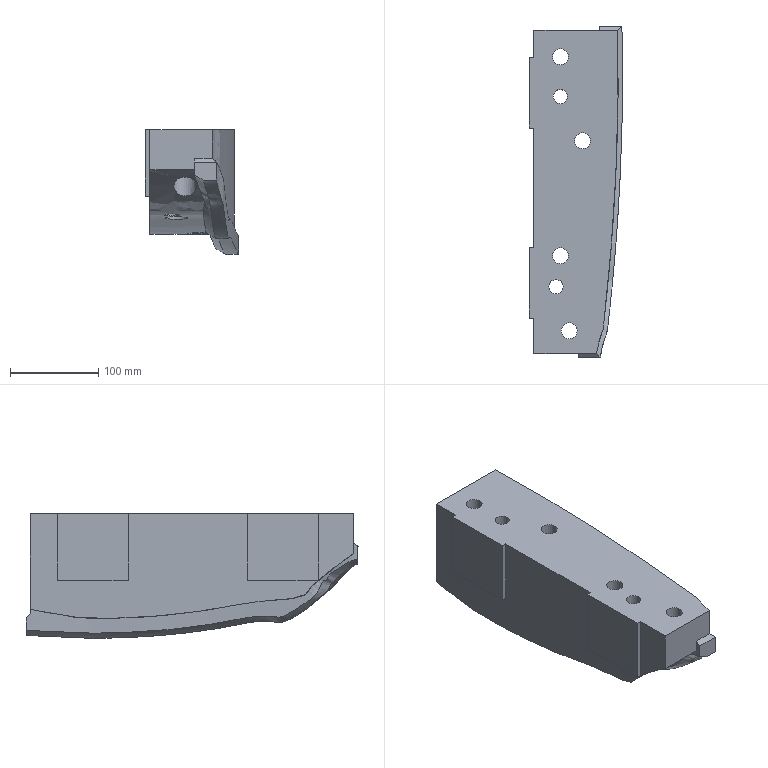Part | NX | features solid 2 | 1 solid | 42 faces | box 105.226 x 375.566 x 140.791 mm | volume 3409460 mm3 | plane 23 | cylinder 12 | spline 7 | commonest cylinder face diameters 18 x6 26 x4 16 x2